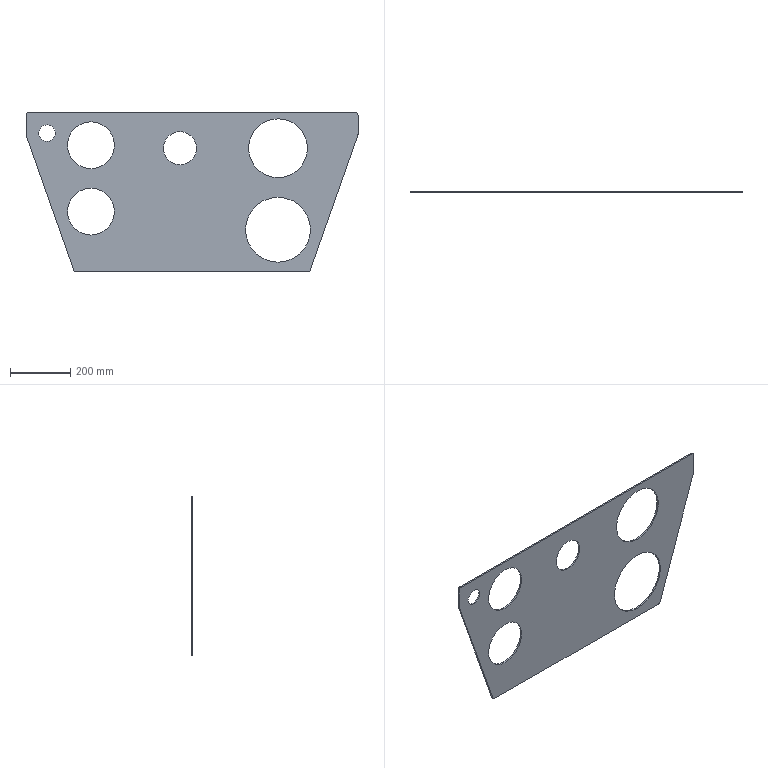Part | SolidWorks | features Fillet 1, FlatPattern 1, ICE 1, SMBaseFlange 1, SheetMetal 1 | 1 solid | 26 faces | box 1100 x 5 x 530 mm | volume 1971755 mm3 | cylinder 18 | plane 8 | commonest cylinder face diameters 20 x6 155 x4 55 x2 110 x2 195 x2 215 x2
STEP:
#1=CARTESIAN_POINT('',(-480.,5.,-97.5));
#2=VERTEX_POINT('',#1);
#3=CARTESIAN_POINT('',(-480.,5.,-42.5));
#4=VERTEX_POINT('',#3);
#5=CARTESIAN_POINT('',(-480.,5.,-70.));
#6=DIRECTION('',(0.,1.,0.));
#7=DIRECTION('',(0.,0.,1.));
#8=AXIS2_PLACEMENT_3D('',#5,#6,#7);
#9=CIRCLE('',#8,27.5);
#10=EDGE_CURVE('',#2,#4,#9,.T.);
#11=ORIENTED_EDGE('',*,*,#10,.T.);
#12=CARTESIAN_POINT('',(-480.,0.,-42.5));
#13=VERTEX_POINT('',#12);
#14=CARTESIAN_POINT('',(-480.,10.,-42.5));
#15=DIRECTION('',(0.,-1.,0.));
#16=VECTOR('',#15,1000.);
#17=LINE('',#14,#16);
#18=EDGE_CURVE('',#4,#13,#17,.T.);
#19=ORIENTED_EDGE('',*,*,#18,.T.);
#20=CARTESIAN_POINT('',(-480.,0.,-97.5));
#21=VERTEX_POINT('',#20);
#22=CARTESIAN_POINT('',(-480.,0.,-70.));
#23=DIRECTION('',(0.,-1.,0.));
#24=DIRECTION('',(0.,0.,-1.));
#25=AXIS2_PLACEMENT_3D('',#22,#23,#24);
#26=CIRCLE('',#25,27.5);
#27=EDGE_CURVE('',#13,#21,#26,.T.);
#28=ORIENTED_EDGE('',*,*,#27,.T.);
#29=CARTESIAN_POINT('',(-480.,10.,-97.5));
#30=DIRECTION('',(0.,-1.,0.));
#31=VECTOR('',#30,1000.);
#32=LINE('',#29,#31);
#33=EDGE_CURVE('',#2,#21,#32,.T.);
#34=ORIENTED_EDGE('',*,*,#33,.F.);
#35=EDGE_LOOP('',(#11,#19,#28,#34));
#36=FACE_OUTER_BOUND('',#35,.T.);
#37=CARTESIAN_POINT('',(-480.,10.,-70.));
#38=DIRECTION('',(0.,-1.,0.));
#39=DIRECTION('',(0.,0.,-1.));
#40=AXIS2_PLACEMENT_3D('',#37,#38,#39);
#41=CYLINDRICAL_SURFACE('',#40,27.5);
#42=ADVANCED_FACE('',(#36),#41,.F.);
#43=CARTESIAN_POINT('',(285.,5.,-497.5));
#44=VERTEX_POINT('',#43);
#45=CARTESIAN_POINT('',(285.,5.,-282.5));
#46=VERTEX_POINT('',#45);
#47=CARTESIAN_POINT('',(285.,5.,-390.));
#48=DIRECTION('',(0.,1.,0.));
#49=DIRECTION('',(0.,0.,1.));
#50=AXIS2_PLACEMENT_3D('',#47,#48,#49);
#51=CIRCLE('',#50,107.5);
#52=EDGE_CURVE('',#44,#46,#51,.T.);
#53=ORIENTED_EDGE('',*,*,#52,.T.);
#54=CARTESIAN_POINT('',(285.,0.,-282.5));
#55=VERTEX_POINT('',#54);
#56=CARTESIAN_POINT('',(285.,10.,-282.5));
#57=DIRECTION('',(0.,-1.,0.));
#58=VECTOR('',#57,1000.);
#59=LINE('',#56,#58);
#60=EDGE_CURVE('',#46,#55,#59,.T.);
#61=ORIENTED_EDGE('',*,*,#60,.T.);
#62=CARTESIAN_POINT('',(285.,0.,-497.5));
#63=VERTEX_POINT('',#62);
#64=CARTESIAN_POINT('',(285.,0.,-390.));
#65=DIRECTION('',(0.,-1.,0.));
#66=DIRECTION('',(0.,0.,-1.));
#67=AXIS2_PLACEMENT_3D('',#64,#65,#66);
#68=CIRCLE('',#67,107.5);
#69=EDGE_CURVE('',#55,#63,#68,.T.);
#70=ORIENTED_EDGE('',*,*,#69,.T.);
#71=CARTESIAN_POINT('',(285.,10.,-497.5));
#72=DIRECTION('',(0.,-1.,0.));
#73=VECTOR('',#72,1000.);
#74=LINE('',#71,#73);
#75=EDGE_CURVE('',#44,#63,#74,.T.);
#76=ORIENTED_EDGE('',*,*,#75,.F.);
#77=EDGE_LOOP('',(#53,#61,#70,#76));
#78=FACE_OUTER_BOUND('',#77,.T.);
#79=CARTESIAN_POINT('',(285.,10.,-390.));
#80=DIRECTION('',(0.,-1.,0.));
#81=DIRECTION('',(0.,0.,-1.));
#82=AXIS2_PLACEMENT_3D('',#79,#80,#81);
#83=CYLINDRICAL_SURFACE('',#82,107.5);
#84=ADVANCED_FACE('',(#78),#83,.F.);
#85=CARTESIAN_POINT('',(285.,5.,-217.5));
#86=VERTEX_POINT('',#85);
#87=CARTESIAN_POINT('',(285.,5.,-22.5));
#88=VERTEX_POINT('',#87);
#89=CARTESIAN_POINT('',(285.,5.,-120.));
#90=DIRECTION('',(0.,1.,0.));
#91=DIRECTION('',(0.,0.,1.));
#92=AXIS2_PLACEMENT_3D('',#89,#90,#91);
#93=CIRCLE('',#92,97.5);
#94=EDGE_CURVE('',#86,#88,#93,.T.);
#95=ORIENTED_EDGE('',*,*,#94,.T.);
#96=CARTESIAN_POINT('',(285.,0.,-22.5));
#97=VERTEX_POINT('',#96);
#98=CARTESIAN_POINT('',(285.,10.,-22.5));
#99=DIRECTION('',(0.,-1.,0.));
#100=VECTOR('',#99,1000.);
#101=LINE('',#98,#100);
#102=EDGE_CURVE('',#88,#97,#101,.T.);
#103=ORIENTED_EDGE('',*,*,#102,.T.);
#104=CARTESIAN_POINT('',(285.,0.,-217.5));
#105=VERTEX_POINT('',#104);
#106=CARTESIAN_POINT('',(285.,0.,-120.));
#107=DIRECTION('',(0.,-1.,0.));
#108=DIRECTION('',(0.,0.,-1.));
#109=AXIS2_PLACEMENT_3D('',#106,#107,#108);
#110=CIRCLE('',#109,97.5);
#111=EDGE_CURVE('',#97,#105,#110,.T.);
#112=ORIENTED_EDGE('',*,*,#111,.T.);
#113=CARTESIAN_POINT('',(285.,10.,-217.5));
#114=DIRECTION('',(0.,-1.,0.));
#115=VECTOR('',#114,1000.);
#116=LINE('',#113,#115);
#117=EDGE_CURVE('',#86,#105,#116,.T.);
#118=ORIENTED_EDGE('',*,*,#117,.F.);
#119=EDGE_LOOP('',(#95,#103,#112,#118));
#120=FACE_OUTER_BOUND('',#119,.T.);
#121=CARTESIAN_POINT('',(285.,10.,-120.));
#122=DIRECTION('',(0.,-1.,0.));
#123=DIRECTION('',(0.,0.,-1.));
#124=AXIS2_PLACEMENT_3D('',#121,#122,#123);
#125=CYLINDRICAL_SURFACE('',#124,97.5);
#126=ADVANCED_FACE('',(#120),#125,.F.);
#127=CARTESIAN_POINT('',(-40.,5.,-175.));
#128=VERTEX_POINT('',#127);
#129=CARTESIAN_POINT('',(-40.,5.,-65.));
#130=VERTEX_POINT('',#129);
#131=CARTESIAN_POINT('',(-40.,5.,-120.));
#132=DIRECTION('',(0.,1.,0.));
#133=DIRECTION('',(0.,0.,1.));
#134=AXIS2_PLACEMENT_3D('',#131,#132,#133);
#135=CIRCLE('',#134,55.);
#136=EDGE_CURVE('',#128,#130,#135,.T.);
#137=ORIENTED_EDGE('',*,*,#136,.T.);
#138=CARTESIAN_POINT('',(-40.,0.,-65.));
#139=VERTEX_POINT('',#138);
#140=CARTESIAN_POINT('',(-40.,10.,-65.));
#141=DIRECTION('',(0.,-1.,0.));
#142=VECTOR('',#141,1000.);
#143=LINE('',#140,#142);
#144=EDGE_CURVE('',#130,#139,#143,.T.);
#145=ORIENTED_EDGE('',*,*,#144,.T.);
#146=CARTESIAN_POINT('',(-40.,0.,-175.));
#147=VERTEX_POINT('',#146);
#148=CARTESIAN_POINT('',(-40.,0.,-120.));
#149=DIRECTION('',(0.,-1.,0.));
#150=DIRECTION('',(0.,0.,-1.));
#151=AXIS2_PLACEMENT_3D('',#148,#149,#150);
#152=CIRCLE('',#151,55.);
#153=EDGE_CURVE('',#139,#147,#152,.T.);
#154=ORIENTED_EDGE('',*,*,#153,.T.);
#155=CARTESIAN_POINT('',(-40.,10.,-175.));
#156=DIRECTION('',(0.,-1.,0.));
#157=VECTOR('',#156,1000.);
#158=LINE('',#155,#157);
#159=EDGE_CURVE('',#128,#147,#158,.T.);
#160=ORIENTED_EDGE('',*,*,#159,.F.);
#161=EDGE_LOOP('',(#137,#145,#154,#160));
#162=FACE_OUTER_BOUND('',#161,.T.);
#163=CARTESIAN_POINT('',(-40.,10.,-120.));
#164=DIRECTION('',(0.,-1.,0.));
#165=DIRECTION('',(0.,0.,-1.));
#166=AXIS2_PLACEMENT_3D('',#163,#164,#165);
#167=CYLINDRICAL_SURFACE('',#166,55.);
#168=ADVANCED_FACE('',(#162),#167,.F.);
#169=CARTESIAN_POINT('',(-335.,5.,-407.5));
#170=VERTEX_POINT('',#169);
#171=CARTESIAN_POINT('',(-335.,5.,-252.5));
#172=VERTEX_POINT('',#171);
#173=CARTESIAN_POINT('',(-335.,5.,-330.));
#174=DIRECTION('',(0.,1.,0.));
#175=DIRECTION('',(0.,0.,1.));
#176=AXIS2_PLACEMENT_3D('',#173,#174,#175);
#177=CIRCLE('',#176,77.5);
#178=EDGE_CURVE('',#170,#172,#177,.T.);
#179=ORIENTED_EDGE('',*,*,#178,.T.);
#180=CARTESIAN_POINT('',(-335.,0.,-252.5));
#181=VERTEX_POINT('',#180);
#182=CARTESIAN_POINT('',(-335.,10.,-252.5));
#183=DIRECTION('',(0.,-1.,0.));
#184=VECTOR('',#183,1000.);
#185=LINE('',#182,#184);
#186=EDGE_CURVE('',#172,#181,#185,.T.);
#187=ORIENTED_EDGE('',*,*,#186,.T.);
#188=CARTESIAN_POINT('',(-335.,0.,-407.5));
#189=VERTEX_POINT('',#188);
#190=CARTESIAN_POINT('',(-335.,0.,-330.));
#191=DIRECTION('',(0.,-1.,0.));
#192=DIRECTION('',(0.,0.,-1.));
#193=AXIS2_PLACEMENT_3D('',#190,#191,#192);
#194=CIRCLE('',#193,77.5);
#195=EDGE_CURVE('',#181,#189,#194,.T.);
#196=ORIENTED_EDGE('',*,*,#195,.T.);
#197=CARTESIAN_POINT('',(-335.,10.,-407.5));
#198=DIRECTION('',(0.,-1.,0.));
#199=VECTOR('',#198,1000.);
#200=LINE('',#197,#199);
#201=EDGE_CURVE('',#170,#189,#200,.T.);
#202=ORIENTED_EDGE('',*,*,#201,.F.);
#203=EDGE_LOOP('',(#179,#187,#196,#202));
#204=FACE_OUTER_BOUND('',#203,.T.);
#205=CARTESIAN_POINT('',(-335.,10.,-330.));
#206=DIRECTION('',(0.,-1.,0.));
#207=DIRECTION('',(0.,0.,-1.));
#208=AXIS2_PLACEMENT_3D('',#205,#206,#207);
#209=CYLINDRICAL_SURFACE('',#208,77.5);
#210=ADVANCED_FACE('',(#204),#209,.F.);
#211=CARTESIAN_POINT('',(-335.,5.,-187.5));
#212=VERTEX_POINT('',#211);
#213=CARTESIAN_POINT('',(-335.,5.,-32.5));
#214=VERTEX_POINT('',#213);
#215=CARTESIAN_POINT('',(-335.,5.,-110.));
#216=DIRECTION('',(0.,1.,0.));
#217=DIRECTION('',(0.,0.,1.));
#218=AXIS2_PLACEMENT_3D('',#215,#216,#217);
#219=CIRCLE('',#218,77.5);
#220=EDGE_CURVE('',#212,#214,#219,.T.);
#221=ORIENTED_EDGE('',*,*,#220,.T.);
#222=CARTESIAN_POINT('',(-335.,0.,-32.5));
#223=VERTEX_POINT('',#222);
#224=CARTESIAN_POINT('',(-335.,10.,-32.5));
#225=DIRECTION('',(0.,-1.,0.));
#226=VECTOR('',#225,1000.);
#227=LINE('',#224,#226);
#228=EDGE_CURVE('',#214,#223,#227,.T.);
#229=ORIENTED_EDGE('',*,*,#228,.T.);
#230=CARTESIAN_POINT('',(-335.,0.,-187.5));
#231=VERTEX_POINT('',#230);
#232=CARTESIAN_POINT('',(-335.,0.,-110.));
#233=DIRECTION('',(0.,-1.,0.));
#234=DIRECTION('',(0.,0.,-1.));
#235=AXIS2_PLACEMENT_3D('',#232,#233,#234);
#236=CIRCLE('',#235,77.5);
#237=EDGE_CURVE('',#223,#231,#236,.T.);
#238=ORIENTED_EDGE('',*,*,#237,.T.);
#239=CARTESIAN_POINT('',(-335.,10.,-187.5));
#240=DIRECTION('',(0.,-1.,0.));
#241=VECTOR('',#240,1000.);
#242=LINE('',#239,#241);
#243=EDGE_CURVE('',#212,#231,#242,.T.);
#244=ORIENTED_EDGE('',*,*,#243,.F.);
#245=EDGE_LOOP('',(#221,#229,#238,#244));
#246=FACE_OUTER_BOUND('',#245,.T.);
#247=CARTESIAN_POINT('',(-335.,10.,-110.));
#248=DIRECTION('',(0.,-1.,0.));
#249=DIRECTION('',(0.,0.,-1.));
#250=AXIS2_PLACEMENT_3D('',#247,#248,#249);
#251=CYLINDRICAL_SURFACE('',#250,77.5);
#252=ADVANCED_FACE('',(#246),#251,.F.);
#253=CARTESIAN_POINT('',(550.,0.,-10.));
#254=VERTEX_POINT('',#253);
#255=CARTESIAN_POINT('',(550.,0.,-73.293));
#256=VERTEX_POINT('',#255);
#257=CARTESIAN_POINT('',(550.,0.,0.));
#258=DIRECTION('',(0.,0.,-1.));
#259=VECTOR('',#258,1000.);
#260=LINE('',#257,#259);
#261=EDGE_CURVE('',#254,#256,#260,.T.);
#262=ORIENTED_EDGE('',*,*,#261,.T.);
#263=CARTESIAN_POINT('',(550.,5.,-73.293));
#264=VERTEX_POINT('',#263);
#265=CARTESIAN_POINT('',(550.,5.,-73.293));
#266=DIRECTION('',(0.,1.,0.));
#267=VECTOR('',#266,1000.);
#268=LINE('',#265,#267);
#269=EDGE_CURVE('',#256,#264,#268,.T.);
#270=ORIENTED_EDGE('',*,*,#269,.T.);
#271=CARTESIAN_POINT('',(550.,5.,-10.));
#272=VERTEX_POINT('',#271);
#273=CARTESIAN_POINT('',(550.,5.,0.));
#274=DIRECTION('',(0.,0.,-1.));
#275=VECTOR('',#274,1000.);
#276=LINE('',#273,#275);
#277=EDGE_CURVE('',#272,#264,#276,.T.);
#278=ORIENTED_EDGE('',*,*,#277,.F.);
#279=CARTESIAN_POINT('',(550.,5.,-10.));
#280=DIRECTION('',(0.,-1.,0.));
#281=VECTOR('',#280,1000.);
#282=LINE('',#279,#281);
#283=EDGE_CURVE('',#272,#254,#282,.T.);
#284=ORIENTED_EDGE('',*,*,#283,.T.);
#285=EDGE_LOOP('',(#262,#270,#278,#284));
#286=FACE_OUTER_BOUND('',#285,.T.);
#287=CARTESIAN_POINT('',(550.,5.,0.));
#288=DIRECTION('',(-1.,0.,0.));
#289=DIRECTION('',(0.,0.,1.));
#290=AXIS2_PLACEMENT_3D('',#287,#288,#289);
#291=PLANE('',#290);
#292=ADVANCED_FACE('',(#286),#291,.F.);
#293=CARTESIAN_POINT('',(549.434,0.,-76.61));
#294=VERTEX_POINT('',#293);
#295=CARTESIAN_POINT('',(392.35,0.,-523.317));
#296=VERTEX_POINT('',#295);
#297=CARTESIAN_POINT('',(550.,0.,-75.));
#298=DIRECTION('',(-0.3317,0.,-0.9434));
#299=VECTOR('',#298,1000.);
#300=LINE('',#297,#299);
#301=EDGE_CURVE('',#294,#296,#300,.T.);
#302=ORIENTED_EDGE('',*,*,#301,.T.);
#303=CARTESIAN_POINT('',(392.35,5.,-523.317));
#304=VERTEX_POINT('',#303);
#305=CARTESIAN_POINT('',(392.35,5.,-523.317));
#306=DIRECTION('',(0.,1.,0.));
#307=VECTOR('',#306,1000.);
#308=LINE('',#305,#307);
#309=EDGE_CURVE('',#296,#304,#308,.T.);
#310=ORIENTED_EDGE('',*,*,#309,.T.);
#311=CARTESIAN_POINT('',(549.434,5.,-76.61));
#312=VERTEX_POINT('',#311);
#313=CARTESIAN_POINT('',(550.,5.,-75.));
#314=DIRECTION('',(-0.3317,0.,-0.9434));
#315=VECTOR('',#314,1000.);
#316=LINE('',#313,#315);
#317=EDGE_CURVE('',#312,#304,#316,.T.);
#318=ORIENTED_EDGE('',*,*,#317,.F.);
#319=CARTESIAN_POINT('',(549.434,5.,-76.61));
#320=DIRECTION('',(0.,-1.,0.));
#321=VECTOR('',#320,1000.);
#322=LINE('',#319,#321);
#323=EDGE_CURVE('',#312,#294,#322,.T.);
#324=ORIENTED_EDGE('',*,*,#323,.T.);
#325=EDGE_LOOP('',(#302,#310,#318,#324));
#326=FACE_OUTER_BOUND('',#325,.T.);
#327=CARTESIAN_POINT('',(550.,5.,-75.));
#328=DIRECTION('',(-0.9434,0.,0.3317));
#329=DIRECTION('',(0.3317,0.,0.9434));
#330=AXIS2_PLACEMENT_3D('',#327,#328,#329);
#331=PLANE('',#330);
#332=ADVANCED_FACE('',(#326),#331,.F.);
#333=CARTESIAN_POINT('',(382.916,0.,-530.));
#334=VERTEX_POINT('',#333);
#335=CARTESIAN_POINT('',(-382.916,0.,-530.));
#336=VERTEX_POINT('',#335);
#337=CARTESIAN_POINT('',(390.,0.,-530.));
#338=DIRECTION('',(-1.,0.,0.));
#339=VECTOR('',#338,1000.);
#340=LINE('',#337,#339);
#341=EDGE_CURVE('',#334,#336,#340,.T.);
#342=ORIENTED_EDGE('',*,*,#341,.T.);
#343=CARTESIAN_POINT('',(-382.916,5.,-530.));
#344=VERTEX_POINT('',#343);
#345=CARTESIAN_POINT('',(-382.916,5.,-530.));
#346=DIRECTION('',(0.,1.,0.));
#347=VECTOR('',#346,1000.);
#348=LINE('',#345,#347);
#349=EDGE_CURVE('',#336,#344,#348,.T.);
#350=ORIENTED_EDGE('',*,*,#349,.T.);
#351=CARTESIAN_POINT('',(382.916,5.,-530.));
#352=VERTEX_POINT('',#351);
#353=CARTESIAN_POINT('',(390.,5.,-530.));
#354=DIRECTION('',(-1.,0.,0.));
#355=VECTOR('',#354,1000.);
#356=LINE('',#353,#355);
#357=EDGE_CURVE('',#352,#344,#356,.T.);
#358=ORIENTED_EDGE('',*,*,#357,.F.);
#359=CARTESIAN_POINT('',(382.916,5.,-530.));
#360=DIRECTION('',(0.,-1.,0.));
#361=VECTOR('',#360,1000.);
#362=LINE('',#359,#361);
#363=EDGE_CURVE('',#352,#334,#362,.T.);
#364=ORIENTED_EDGE('',*,*,#363,.T.);
#365=EDGE_LOOP('',(#342,#350,#358,#364));
#366=FACE_OUTER_BOUND('',#365,.T.);
#367=CARTESIAN_POINT('',(390.,5.,-530.));
#368=DIRECTION('',(0.,0.,1.));
#369=DIRECTION('',(1.,0.,0.));
#370=AXIS2_PLACEMENT_3D('',#367,#368,#369);
#371=PLANE('',#370);
#372=ADVANCED_FACE('',(#366),#371,.F.);
#373=CARTESIAN_POINT('',(-392.35,0.,-523.317));
#374=VERTEX_POINT('',#373);
#375=CARTESIAN_POINT('',(-549.434,0.,-76.61));
#376=VERTEX_POINT('',#375);
#377=CARTESIAN_POINT('',(-550.,0.,-75.));
#378=DIRECTION('',(-0.3317,0.,0.9434));
#379=VECTOR('',#378,1000.);
#380=LINE('',#377,#379);
#381=EDGE_CURVE('',#374,#376,#380,.T.);
#382=ORIENTED_EDGE('',*,*,#381,.T.);
#383=CARTESIAN_POINT('',(-549.434,5.,-76.61));
#384=VERTEX_POINT('',#383);
#385=CARTESIAN_POINT('',(-549.434,5.,-76.61));
#386=DIRECTION('',(0.,1.,0.));
#387=VECTOR('',#386,1000.);
#388=LINE('',#385,#387);
#389=EDGE_CURVE('',#376,#384,#388,.T.);
#390=ORIENTED_EDGE('',*,*,#389,.T.);
#391=CARTESIAN_POINT('',(-392.35,5.,-523.317));
#392=VERTEX_POINT('',#391);
#393=CARTESIAN_POINT('',(-550.,5.,-75.));
#394=DIRECTION('',(-0.3317,0.,0.9434));
#395=VECTOR('',#394,1000.);
#396=LINE('',#393,#395);
#397=EDGE_CURVE('',#392,#384,#396,.T.);
#398=ORIENTED_EDGE('',*,*,#397,.F.);
#399=CARTESIAN_POINT('',(-392.35,5.,-523.317));
#400=DIRECTION('',(0.,-1.,0.));
#401=VECTOR('',#400,1000.);
#402=LINE('',#399,#401);
#403=EDGE_CURVE('',#392,#374,#402,.T.);
#404=ORIENTED_EDGE('',*,*,#403,.T.);
#405=EDGE_LOOP('',(#382,#390,#398,#404));
#406=FACE_OUTER_BOUND('',#405,.T.);
#407=CARTESIAN_POINT('',(-550.,5.,-75.));
#408=DIRECTION('',(0.9434,0.,0.3317));
#409=DIRECTION('',(0.3317,0.,-0.9434));
#410=AXIS2_PLACEMENT_3D('',#407,#408,#409);
#411=PLANE('',#410);
#412=ADVANCED_FACE('',(#406),#411,.F.);
#413=CARTESIAN_POINT('',(-550.,0.,-73.293));
#414=VERTEX_POINT('',#413);
#415=CARTESIAN_POINT('',(-550.,0.,-10.));
#416=VERTEX_POINT('',#415);
#417=CARTESIAN_POINT('',(-550.,0.,0.));
#418=DIRECTION('',(0.,0.,1.));
#419=VECTOR('',#418,1000.);
#420=LINE('',#417,#419);
#421=EDGE_CURVE('',#414,#416,#420,.T.);
#422=ORIENTED_EDGE('',*,*,#421,.T.);
#423=CARTESIAN_POINT('',(-550.,5.,-10.));
#424=VERTEX_POINT('',#423);
#425=CARTESIAN_POINT('',(-550.,5.,-10.));
#426=DIRECTION('',(0.,1.,0.));
#427=VECTOR('',#426,1000.);
#428=LINE('',#425,#427);
#429=EDGE_CURVE('',#416,#424,#428,.T.);
#430=ORIENTED_EDGE('',*,*,#429,.T.);
#431=CARTESIAN_POINT('',(-550.,5.,-73.293));
#432=VERTEX_POINT('',#431);
#433=CARTESIAN_POINT('',(-550.,5.,0.));
#434=DIRECTION('',(0.,0.,1.));
#435=VECTOR('',#434,1000.);
#436=LINE('',#433,#435);
#437=EDGE_CURVE('',#432,#424,#436,.T.);
#438=ORIENTED_EDGE('',*,*,#437,.F.);
#439=CARTESIAN_POINT('',(-550.,5.,-73.293));
#440=DIRECTION('',(0.,-1.,0.));
#441=VECTOR('',#440,1000.);
#442=LINE('',#439,#441);
#443=EDGE_CURVE('',#432,#414,#442,.T.);
#444=ORIENTED_EDGE('',*,*,#443,.T.);
#445=EDGE_LOOP('',(#422,#430,#438,#444));
#446=FACE_OUTER_BOUND('',#445,.T.);
#447=CARTESIAN_POINT('',(-550.,5.,0.));
#448=DIRECTION('',(1.,0.,0.));
#449=DIRECTION('',(0.,0.,-1.));
#450=AXIS2_PLACEMENT_3D('',#447,#448,#449);
#451=PLANE('',#450);
#452=ADVANCED_FACE('',(#446),#451,.F.);
#453=CARTESIAN_POINT('',(-540.,5.,0.));
#454=VERTEX_POINT('',#453);
#455=CARTESIAN_POINT('',(540.,5.,0.));
#456=VERTEX_POINT('',#455);
#457=CARTESIAN_POINT('',(-550.,5.,0.));
#458=DIRECTION('',(1.,0.,0.));
#459=VECTOR('',#458,1000.);
#460=LINE('',#457,#459);
#461=EDGE_CURVE('',#454,#456,#460,.T.);
#462=ORIENTED_EDGE('',*,*,#461,.F.);
#463=CARTESIAN_POINT('',(-540.,0.,0.));
#464=VERTEX_POINT('',#463);
#465=CARTESIAN_POINT('',(-540.,5.,0.));
#466=DIRECTION('',(0.,-1.,0.));
#467=VECTOR('',#466,1000.);
#468=LINE('',#465,#467);
#469=EDGE_CURVE('',#454,#464,#468,.T.);
#470=ORIENTED_EDGE('',*,*,#469,.T.);
#471=CARTESIAN_POINT('',(540.,0.,0.));
#472=VERTEX_POINT('',#471);
#473=CARTESIAN_POINT('',(-550.,0.,0.));
#474=DIRECTION('',(1.,0.,0.));
#475=VECTOR('',#474,1000.);
#476=LINE('',#473,#475);
#477=EDGE_CURVE('',#464,#472,#476,.T.);
#478=ORIENTED_EDGE('',*,*,#477,.T.);
#479=CARTESIAN_POINT('',(540.,5.,0.));
#480=DIRECTION('',(0.,1.,0.));
#481=VECTOR('',#480,1000.);
#482=LINE('',#479,#481);
#483=EDGE_CURVE('',#472,#456,#482,.T.);
#484=ORIENTED_EDGE('',*,*,#483,.T.);
#485=EDGE_LOOP('',(#462,#470,#478,#484));
#486=FACE_OUTER_BOUND('',#485,.T.);
#487=CARTESIAN_POINT('',(-550.,5.,0.));
#488=DIRECTION('',(0.,0.,-1.));
#489=DIRECTION('',(-1.,0.,0.));
#490=AXIS2_PLACEMENT_3D('',#487,#488,#489);
#491=PLANE('',#490);
#492=ADVANCED_FACE('',(#486),#491,.F.);
#493=ORIENTED_EDGE('',*,*,#10,.F.);
#494=CARTESIAN_POINT('',(-480.,5.,-70.));
#495=DIRECTION('',(0.,1.,0.));
#496=DIRECTION('',(0.,0.,1.));
#497=AXIS2_PLACEMENT_3D('',#494,#495,#496);
#498=CIRCLE('',#497,27.5);
#499=EDGE_CURVE('',#4,#2,#498,.T.);
#500=ORIENTED_EDGE('',*,*,#499,.F.);
#501=EDGE_LOOP('',(#493,#500));
#502=FACE_BOUND('',#501,.T.);
#503=ORIENTED_EDGE('',*,*,#52,.F.);
#504=CARTESIAN_POINT('',(285.,5.,-390.));
#505=DIRECTION('',(0.,1.,0.));
#506=DIRECTION('',(0.,0.,1.));
#507=AXIS2_PLACEMENT_3D('',#504,#505,#506);
#508=CIRCLE('',#507,107.5);
#509=EDGE_CURVE('',#46,#44,#508,.T.);
#510=ORIENTED_EDGE('',*,*,#509,.F.);
#511=EDGE_LOOP('',(#503,#510));
#512=FACE_BOUND('',#511,.T.);
#513=ORIENTED_EDGE('',*,*,#94,.F.);
#514=CARTESIAN_POINT('',(285.,5.,-120.));
#515=DIRECTION('',(0.,1.,0.));
#516=DIRECTION('',(0.,0.,1.));
#517=AXIS2_PLACEMENT_3D('',#514,#515,#516);
#518=CIRCLE('',#517,97.5);
#519=EDGE_CURVE('',#88,#86,#518,.T.);
#520=ORIENTED_EDGE('',*,*,#519,.F.);
#521=EDGE_LOOP('',(#513,#520));
#522=FACE_BOUND('',#521,.T.);
#523=ORIENTED_EDGE('',*,*,#136,.F.);
#524=CARTESIAN_POINT('',(-40.,5.,-120.));
#525=DIRECTION('',(0.,1.,0.));
#526=DIRECTION('',(0.,0.,1.));
#527=AXIS2_PLACEMENT_3D('',#524,#525,#526);
#528=CIRCLE('',#527,55.);
#529=EDGE_CURVE('',#130,#128,#528,.T.);
#530=ORIENTED_EDGE('',*,*,#529,.F.);
#531=EDGE_LOOP('',(#523,#530));
#532=FACE_BOUND('',#531,.T.);
#533=ORIENTED_EDGE('',*,*,#178,.F.);
#534=CARTESIAN_POINT('',(-335.,5.,-330.));
#535=DIRECTION('',(0.,1.,0.));
#536=DIRECTION('',(0.,0.,1.));
#537=AXIS2_PLACEMENT_3D('',#534,#535,#536);
#538=CIRCLE('',#537,77.5);
#539=EDGE_CURVE('',#172,#170,#538,.T.);
#540=ORIENTED_EDGE('',*,*,#539,.F.);
#541=EDGE_LOOP('',(#533,#540));
#542=FACE_BOUND('',#541,.T.);
#543=ORIENTED_EDGE('',*,*,#220,.F.);
#544=CARTESIAN_POINT('',(-335.,5.,-110.));
#545=DIRECTION('',(0.,1.,0.));
#546=DIRECTION('',(0.,0.,1.));
#547=AXIS2_PLACEMENT_3D('',#544,#545,#546);
#548=CIRCLE('',#547,77.5);
#549=EDGE_CURVE('',#214,#212,#548,.T.);
#550=ORIENTED_EDGE('',*,*,#549,.F.);
#551=EDGE_LOOP('',(#543,#550));
#552=FACE_BOUND('',#551,.T.);
#553=ORIENTED_EDGE('',*,*,#437,.T.);
#554=CARTESIAN_POINT('',(-540.,5.,-10.));
#555=DIRECTION('',(0.,1.,0.));
#556=DIRECTION('',(0.,0.,1.));
#557=AXIS2_PLACEMENT_3D('',#554,#555,#556);
#558=CIRCLE('',#557,10.);
#559=EDGE_CURVE('',#424,#454,#558,.T.);
#560=ORIENTED_EDGE('',*,*,#559,.T.);
#561=ORIENTED_EDGE('',*,*,#461,.T.);
#562=CARTESIAN_POINT('',(540.,5.,-10.));
#563=DIRECTION('',(0.,1.,0.));
#564=DIRECTION('',(0.,0.,1.));
#565=AXIS2_PLACEMENT_3D('',#562,#563,#564);
#566=CIRCLE('',#565,10.);
#567=EDGE_CURVE('',#456,#272,#566,.T.);
#568=ORIENTED_EDGE('',*,*,#567,.T.);
#569=ORIENTED_EDGE('',*,*,#277,.T.);
#570=CARTESIAN_POINT('',(540.,5.,-73.293));
#571=DIRECTION('',(0.,1.,0.));
#572=DIRECTION('',(0.,0.,1.));
#573=AXIS2_PLACEMENT_3D('',#570,#571,#572);
#574=CIRCLE('',#573,10.);
#575=EDGE_CURVE('',#264,#312,#574,.T.);
#576=ORIENTED_EDGE('',*,*,#575,.T.);
#577=ORIENTED_EDGE('',*,*,#317,.T.);
#578=CARTESIAN_POINT('',(382.916,5.,-520.));
#579=DIRECTION('',(0.,1.,0.));
#580=DIRECTION('',(0.,0.,1.));
#581=AXIS2_PLACEMENT_3D('',#578,#579,#580);
#582=CIRCLE('',#581,10.);
#583=EDGE_CURVE('',#304,#352,#582,.T.);
#584=ORIENTED_EDGE('',*,*,#583,.T.);
#585=ORIENTED_EDGE('',*,*,#357,.T.);
#586=CARTESIAN_POINT('',(-382.916,5.,-520.));
#587=DIRECTION('',(0.,1.,0.));
#588=DIRECTION('',(0.,0.,1.));
#589=AXIS2_PLACEMENT_3D('',#586,#587,#588);
#590=CIRCLE('',#589,10.);
#591=EDGE_CURVE('',#344,#392,#590,.T.);
#592=ORIENTED_EDGE('',*,*,#591,.T.);
#593=ORIENTED_EDGE('',*,*,#397,.T.);
#594=CARTESIAN_POINT('',(-540.,5.,-73.293));
#595=DIRECTION('',(0.,1.,0.));
#596=DIRECTION('',(0.,0.,1.));
#597=AXIS2_PLACEMENT_3D('',#594,#595,#596);
#598=CIRCLE('',#597,10.);
#599=EDGE_CURVE('',#384,#432,#598,.T.);
#600=ORIENTED_EDGE('',*,*,#599,.T.);
#601=EDGE_LOOP('',(#553,#560,#561,#568,#569,#576,#577,#584,#585,#592,#593,#600));
#602=FACE_OUTER_BOUND('',#601,.T.);
#603=CARTESIAN_POINT('',(0.,5.,0.));
#604=DIRECTION('',(0.,1.,0.));
#605=DIRECTION('',(0.,0.,1.));
#606=AXIS2_PLACEMENT_3D('',#603,#604,#605);
#607=PLANE('',#606);
#608=ADVANCED_FACE('',(#502,#512,#522,#532,#542,#552,#602),#607,.T.);
#609=CARTESIAN_POINT('',(-480.,0.,-70.));
#610=DIRECTION('',(0.,-1.,0.));
#611=DIRECTION('',(0.,0.,-1.));
#612=AXIS2_PLACEMENT_3D('',#609,#610,#611);
#613=CIRCLE('',#612,27.5);
#614=EDGE_CURVE('',#21,#13,#613,.T.);
#615=ORIENTED_EDGE('',*,*,#614,.F.);
#616=ORIENTED_EDGE('',*,*,#27,.F.);
#617=EDGE_LOOP('',(#615,#616));
#618=FACE_BOUND('',#617,.T.);
#619=CARTESIAN_POINT('',(285.,0.,-390.));
#620=DIRECTION('',(0.,-1.,0.));
#621=DIRECTION('',(0.,0.,-1.));
#622=AXIS2_PLACEMENT_3D('',#619,#620,#621);
#623=CIRCLE('',#622,107.5);
#624=EDGE_CURVE('',#63,#55,#623,.T.);
#625=ORIENTED_EDGE('',*,*,#624,.F.);
#626=ORIENTED_EDGE('',*,*,#69,.F.);
#627=EDGE_LOOP('',(#625,#626));
#628=FACE_BOUND('',#627,.T.);
#629=CARTESIAN_POINT('',(285.,0.,-120.));
#630=DIRECTION('',(0.,-1.,0.));
#631=DIRECTION('',(0.,0.,-1.));
#632=AXIS2_PLACEMENT_3D('',#629,#630,#631);
#633=CIRCLE('',#632,97.5);
#634=EDGE_CURVE('',#105,#97,#633,.T.);
#635=ORIENTED_EDGE('',*,*,#634,.F.);
#636=ORIENTED_EDGE('',*,*,#111,.F.);
#637=EDGE_LOOP('',(#635,#636));
#638=FACE_BOUND('',#637,.T.);
#639=CARTESIAN_POINT('',(-40.,0.,-120.));
#640=DIRECTION('',(0.,-1.,0.));
#641=DIRECTION('',(0.,0.,-1.));
#642=AXIS2_PLACEMENT_3D('',#639,#640,#641);
#643=CIRCLE('',#642,55.);
#644=EDGE_CURVE('',#147,#139,#643,.T.);
#645=ORIENTED_EDGE('',*,*,#644,.F.);
#646=ORIENTED_EDGE('',*,*,#153,.F.);
#647=EDGE_LOOP('',(#645,#646));
#648=FACE_BOUND('',#647,.T.);
#649=CARTESIAN_POINT('',(-335.,0.,-330.));
#650=DIRECTION('',(0.,-1.,0.));
#651=DIRECTION('',(0.,0.,-1.));
#652=AXIS2_PLACEMENT_3D('',#649,#650,#651);
#653=CIRCLE('',#652,77.5);
#654=EDGE_CURVE('',#189,#181,#653,.T.);
#655=ORIENTED_EDGE('',*,*,#654,.F.);
#656=ORIENTED_EDGE('',*,*,#195,.F.);
#657=EDGE_LOOP('',(#655,#656));
#658=FACE_BOUND('',#657,.T.);
#659=CARTESIAN_POINT('',(-335.,0.,-110.));
#660=DIRECTION('',(0.,-1.,0.));
#661=DIRECTION('',(0.,0.,-1.));
#662=AXIS2_PLACEMENT_3D('',#659,#660,#661);
#663=CIRCLE('',#662,77.5);
#664=EDGE_CURVE('',#231,#223,#663,.T.);
#665=ORIENTED_EDGE('',*,*,#664,.F.);
#666=ORIENTED_EDGE('',*,*,#237,.F.);
#667=EDGE_LOOP('',(#665,#666));
#668=FACE_BOUND('',#667,.T.);
#669=ORIENTED_EDGE('',*,*,#477,.F.);
#670=CARTESIAN_POINT('',(-540.,0.,-10.));
#671=DIRECTION('',(0.,-1.,0.));
#672=DIRECTION('',(0.,0.,1.));
#673=AXIS2_PLACEMENT_3D('',#670,#671,#672);
#674=CIRCLE('',#673,10.);
#675=EDGE_CURVE('',#464,#416,#674,.T.);
#676=ORIENTED_EDGE('',*,*,#675,.T.);
#677=ORIENTED_EDGE('',*,*,#421,.F.);
#678=CARTESIAN_POINT('',(-540.,0.,-73.293));
#679=DIRECTION('',(0.,-1.,0.));
#680=DIRECTION('',(0.,0.,1.));
#681=AXIS2_PLACEMENT_3D('',#678,#679,#680);
#682=CIRCLE('',#681,10.);
#683=EDGE_CURVE('',#414,#376,#682,.T.);
#684=ORIENTED_EDGE('',*,*,#683,.T.);
#685=ORIENTED_EDGE('',*,*,#381,.F.);
#686=CARTESIAN_POINT('',(-382.916,0.,-520.));
#687=DIRECTION('',(0.,-1.,0.));
#688=DIRECTION('',(0.,0.,1.));
#689=AXIS2_PLACEMENT_3D('',#686,#687,#688);
#690=CIRCLE('',#689,10.);
#691=EDGE_CURVE('',#374,#336,#690,.T.);
#692=ORIENTED_EDGE('',*,*,#691,.T.);
#693=ORIENTED_EDGE('',*,*,#341,.F.);
#694=CARTESIAN_POINT('',(382.916,0.,-520.));
#695=DIRECTION('',(0.,-1.,0.));
#696=DIRECTION('',(0.,0.,1.));
#697=AXIS2_PLACEMENT_3D('',#694,#695,#696);
#698=CIRCLE('',#697,10.);
#699=EDGE_CURVE('',#334,#296,#698,.T.);
#700=ORIENTED_EDGE('',*,*,#699,.T.);
#701=ORIENTED_EDGE('',*,*,#301,.F.);
#702=CARTESIAN_POINT('',(540.,0.,-73.293));
#703=DIRECTION('',(0.,-1.,0.));
#704=DIRECTION('',(0.,0.,1.));
#705=AXIS2_PLACEMENT_3D('',#702,#703,#704);
#706=CIRCLE('',#705,10.);
#707=EDGE_CURVE('',#294,#256,#706,.T.);
#708=ORIENTED_EDGE('',*,*,#707,.T.);
#709=ORIENTED_EDGE('',*,*,#261,.F.);
#710=CARTESIAN_POINT('',(540.,0.,-10.));
#711=DIRECTION('',(0.,-1.,0.));
#712=DIRECTION('',(0.,0.,1.));
#713=AXIS2_PLACEMENT_3D('',#710,#711,#712);
#714=CIRCLE('',#713,10.);
#715=EDGE_CURVE('',#254,#472,#714,.T.);
#716=ORIENTED_EDGE('',*,*,#715,.T.);
#717=EDGE_LOOP('',(#669,#676,#677,#684,#685,#692,#693,#700,#701,#708,#709,#716));
#718=FACE_OUTER_BOUND('',#717,.T.);
#719=CARTESIAN_POINT('',(0.,0.,0.));
#720=DIRECTION('',(0.,1.,0.));
#721=DIRECTION('',(0.,0.,1.));
#722=AXIS2_PLACEMENT_3D('',#719,#720,#721);
#723=PLANE('',#722);
#724=ADVANCED_FACE('',(#618,#628,#638,#648,#658,#668,#718),#723,.F.);
#725=ORIENTED_EDGE('',*,*,#228,.F.);
#726=ORIENTED_EDGE('',*,*,#549,.T.);
#727=ORIENTED_EDGE('',*,*,#243,.T.);
#728=ORIENTED_EDGE('',*,*,#664,.T.);
#729=EDGE_LOOP('',(#725,#726,#727,#728));
#730=FACE_OUTER_BOUND('',#729,.T.);
#731=CARTESIAN_POINT('',(-335.,10.,-110.));
#732=DIRECTION('',(0.,-1.,0.));
#733=DIRECTION('',(0.,0.,-1.));
#734=AXIS2_PLACEMENT_3D('',#731,#732,#733);
#735=CYLINDRICAL_SURFACE('',#734,77.5);
#736=ADVANCED_FACE('',(#730),#735,.F.);
#737=ORIENTED_EDGE('',*,*,#186,.F.);
#738=ORIENTED_EDGE('',*,*,#539,.T.);
#739=ORIENTED_EDGE('',*,*,#201,.T.);
#740=ORIENTED_EDGE('',*,*,#654,.T.);
#741=EDGE_LOOP('',(#737,#738,#739,#740));
#742=FACE_OUTER_BOUND('',#741,.T.);
#743=CARTESIAN_POINT('',(-335.,10.,-330.));
#744=DIRECTION('',(0.,-1.,0.));
#745=DIRECTION('',(0.,0.,-1.));
#746=AXIS2_PLACEMENT_3D('',#743,#744,#745);
#747=CYLINDRICAL_SURFACE('',#746,77.5);
#748=ADVANCED_FACE('',(#742),#747,.F.);
#749=ORIENTED_EDGE('',*,*,#144,.F.);
#750=ORIENTED_EDGE('',*,*,#529,.T.);
#751=ORIENTED_EDGE('',*,*,#159,.T.);
#752=ORIENTED_EDGE('',*,*,#644,.T.);
#753=EDGE_LOOP('',(#749,#750,#751,#752));
#754=FACE_OUTER_BOUND('',#753,.T.);
#755=CARTESIAN_POINT('',(-40.,10.,-120.));
#756=DIRECTION('',(0.,-1.,0.));
#757=DIRECTION('',(0.,0.,-1.));
#758=AXIS2_PLACEMENT_3D('',#755,#756,#757);
#759=CYLINDRICAL_SURFACE('',#758,55.);
#760=ADVANCED_FACE('',(#754),#759,.F.);
#761=ORIENTED_EDGE('',*,*,#102,.F.);
#762=ORIENTED_EDGE('',*,*,#519,.T.);
#763=ORIENTED_EDGE('',*,*,#117,.T.);
#764=ORIENTED_EDGE('',*,*,#634,.T.);
#765=EDGE_LOOP('',(#761,#762,#763,#764));
#766=FACE_OUTER_BOUND('',#765,.T.);
#767=CARTESIAN_POINT('',(285.,10.,-120.));
#768=DIRECTION('',(0.,-1.,0.));
#769=DIRECTION('',(0.,0.,-1.));
#770=AXIS2_PLACEMENT_3D('',#767,#768,#769);
#771=CYLINDRICAL_SURFACE('',#770,97.5);
#772=ADVANCED_FACE('',(#766),#771,.F.);
#773=ORIENTED_EDGE('',*,*,#60,.F.);
#774=ORIENTED_EDGE('',*,*,#509,.T.);
#775=ORIENTED_EDGE('',*,*,#75,.T.);
#776=ORIENTED_EDGE('',*,*,#624,.T.);
#777=EDGE_LOOP('',(#773,#774,#775,#776));
#778=FACE_OUTER_BOUND('',#777,.T.);
#779=CARTESIAN_POINT('',(285.,10.,-390.));
#780=DIRECTION('',(0.,-1.,0.));
#781=DIRECTION('',(0.,0.,-1.));
#782=AXIS2_PLACEMENT_3D('',#779,#780,#781);
#783=CYLINDRICAL_SURFACE('',#782,107.5);
#784=ADVANCED_FACE('',(#778),#783,.F.);
#785=ORIENTED_EDGE('',*,*,#18,.F.);
#786=ORIENTED_EDGE('',*,*,#499,.T.);
#787=ORIENTED_EDGE('',*,*,#33,.T.);
#788=ORIENTED_EDGE('',*,*,#614,.T.);
#789=EDGE_LOOP('',(#785,#786,#787,#788));
#790=FACE_OUTER_BOUND('',#789,.T.);
#791=CARTESIAN_POINT('',(-480.,10.,-70.));
#792=DIRECTION('',(0.,-1.,0.));
#793=DIRECTION('',(0.,0.,-1.));
#794=AXIS2_PLACEMENT_3D('',#791,#792,#793);
#795=CYLINDRICAL_SURFACE('',#794,27.5);
#796=ADVANCED_FACE('',(#790),#795,.F.);
#797=ORIENTED_EDGE('',*,*,#559,.F.);
#798=ORIENTED_EDGE('',*,*,#429,.F.);
#799=ORIENTED_EDGE('',*,*,#675,.F.);
#800=ORIENTED_EDGE('',*,*,#469,.F.);
#801=EDGE_LOOP('',(#797,#798,#799,#800));
#802=FACE_OUTER_BOUND('',#801,.T.);
#803=CARTESIAN_POINT('',(-540.,5.,-10.));
#804=DIRECTION('',(0.,-1.,0.));
#805=DIRECTION('',(0.,0.,-1.));
#806=AXIS2_PLACEMENT_3D('',#803,#804,#805);
#807=CYLINDRICAL_SURFACE('',#806,10.);
#808=ADVANCED_FACE('',(#802),#807,.T.);
#809=ORIENTED_EDGE('',*,*,#599,.F.);
#810=ORIENTED_EDGE('',*,*,#389,.F.);
#811=ORIENTED_EDGE('',*,*,#683,.F.);
#812=ORIENTED_EDGE('',*,*,#443,.F.);
#813=EDGE_LOOP('',(#809,#810,#811,#812));
#814=FACE_OUTER_BOUND('',#813,.T.);
#815=CARTESIAN_POINT('',(-540.,5.,-73.293));
#816=DIRECTION('',(0.,-1.,0.));
#817=DIRECTION('',(0.,0.,-1.));
#818=AXIS2_PLACEMENT_3D('',#815,#816,#817);
#819=CYLINDRICAL_SURFACE('',#818,10.);
#820=ADVANCED_FACE('',(#814),#819,.T.);
#821=ORIENTED_EDGE('',*,*,#591,.F.);
#822=ORIENTED_EDGE('',*,*,#349,.F.);
#823=ORIENTED_EDGE('',*,*,#691,.F.);
#824=ORIENTED_EDGE('',*,*,#403,.F.);
#825=EDGE_LOOP('',(#821,#822,#823,#824));
#826=FACE_OUTER_BOUND('',#825,.T.);
#827=CARTESIAN_POINT('',(-382.916,5.,-520.));
#828=DIRECTION('',(0.,-1.,0.));
#829=DIRECTION('',(0.,0.,-1.));
#830=AXIS2_PLACEMENT_3D('',#827,#828,#829);
#831=CYLINDRICAL_SURFACE('',#830,10.);
#832=ADVANCED_FACE('',(#826),#831,.T.);
#833=ORIENTED_EDGE('',*,*,#583,.F.);
#834=ORIENTED_EDGE('',*,*,#309,.F.);
#835=ORIENTED_EDGE('',*,*,#699,.F.);
#836=ORIENTED_EDGE('',*,*,#363,.F.);
#837=EDGE_LOOP('',(#833,#834,#835,#836));
#838=FACE_OUTER_BOUND('',#837,.T.);
#839=CARTESIAN_POINT('',(382.916,5.,-520.));
#840=DIRECTION('',(0.,-1.,0.));
#841=DIRECTION('',(0.,0.,-1.));
#842=AXIS2_PLACEMENT_3D('',#839,#840,#841);
#843=CYLINDRICAL_SURFACE('',#842,10.);
#844=ADVANCED_FACE('',(#838),#843,.T.);
#845=ORIENTED_EDGE('',*,*,#575,.F.);
#846=ORIENTED_EDGE('',*,*,#269,.F.);
#847=ORIENTED_EDGE('',*,*,#707,.F.);
#848=ORIENTED_EDGE('',*,*,#323,.F.);
#849=EDGE_LOOP('',(#845,#846,#847,#848));
#850=FACE_OUTER_BOUND('',#849,.T.);
#851=CARTESIAN_POINT('',(540.,5.,-73.293));
#852=DIRECTION('',(0.,-1.,0.));
#853=DIRECTION('',(0.,0.,-1.));
#854=AXIS2_PLACEMENT_3D('',#851,#852,#853);
#855=CYLINDRICAL_SURFACE('',#854,10.);
#856=ADVANCED_FACE('',(#850),#855,.T.);
#857=ORIENTED_EDGE('',*,*,#567,.F.);
#858=ORIENTED_EDGE('',*,*,#483,.F.);
#859=ORIENTED_EDGE('',*,*,#715,.F.);
#860=ORIENTED_EDGE('',*,*,#283,.F.);
#861=EDGE_LOOP('',(#857,#858,#859,#860));
#862=FACE_OUTER_BOUND('',#861,.T.);
#863=CARTESIAN_POINT('',(540.,5.,-10.));
#864=DIRECTION('',(0.,-1.,0.));
#865=DIRECTION('',(0.,0.,-1.));
#866=AXIS2_PLACEMENT_3D('',#863,#864,#865);
#867=CYLINDRICAL_SURFACE('',#866,10.);
#868=ADVANCED_FACE('',(#862),#867,.T.);
#869=CLOSED_SHELL('',(#42,#84,#126,#168,#210,#252,#292,#332,#372,#412,#452,#492,#608,#724,#736,#748,#760,#772,#784,#796,#808,#820,#832,#844,#856,#868));
#870=MANIFOLD_SOLID_BREP('',#869);
#871=CARTESIAN_POINT('',(0.,0.,0.));
#872=DIRECTION('',(0.,0.,1.));
#873=DIRECTION('',(1.,0.,0.));
#874=AXIS2_PLACEMENT_3D('',#871,#872,#873);
#875=(LENGTH_UNIT()NAMED_UNIT(*)SI_UNIT(.MILLI.,.METRE.));
#876=UNCERTAINTY_MEASURE_WITH_UNIT(LENGTH_MEASURE(0.00001),#875,'','');
#877=(NAMED_UNIT(*)PLANE_ANGLE_UNIT()SI_UNIT($,.RADIAN.));
#878=(NAMED_UNIT(*)SI_UNIT($,.STERADIAN.)SOLID_ANGLE_UNIT());
#879=(GEOMETRIC_REPRESENTATION_CONTEXT(3)GLOBAL_UNCERTAINTY_ASSIGNED_CONTEXT((#876))GLOBAL_UNIT_ASSIGNED_CONTEXT((#875,#877,#878))REPRESENTATION_CONTEXT('',''));
#880=ADVANCED_BREP_SHAPE_REPRESENTATION('',(#870,#874),#879);